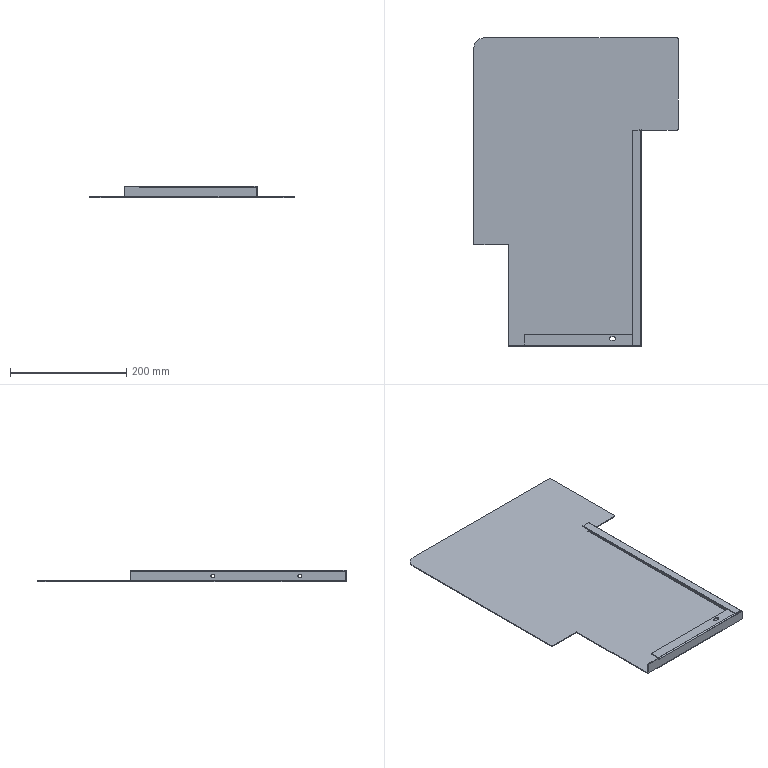Part | SolidWorks | features ICE 4, EdgeFlange 3, Fillet 1, FlatPattern 1, SMBaseFlange 1, SMMiteredFlange 1, SheetMetal 1 | 1 solid | 68 faces | box 352 x 531.5 x 20 mm | volume 257244 mm3 | plane 47 | cylinder 21 | commonest cylinder face diameters 1 x4 4 x4 6.4 x4 3 x3 6 x3 13 x2